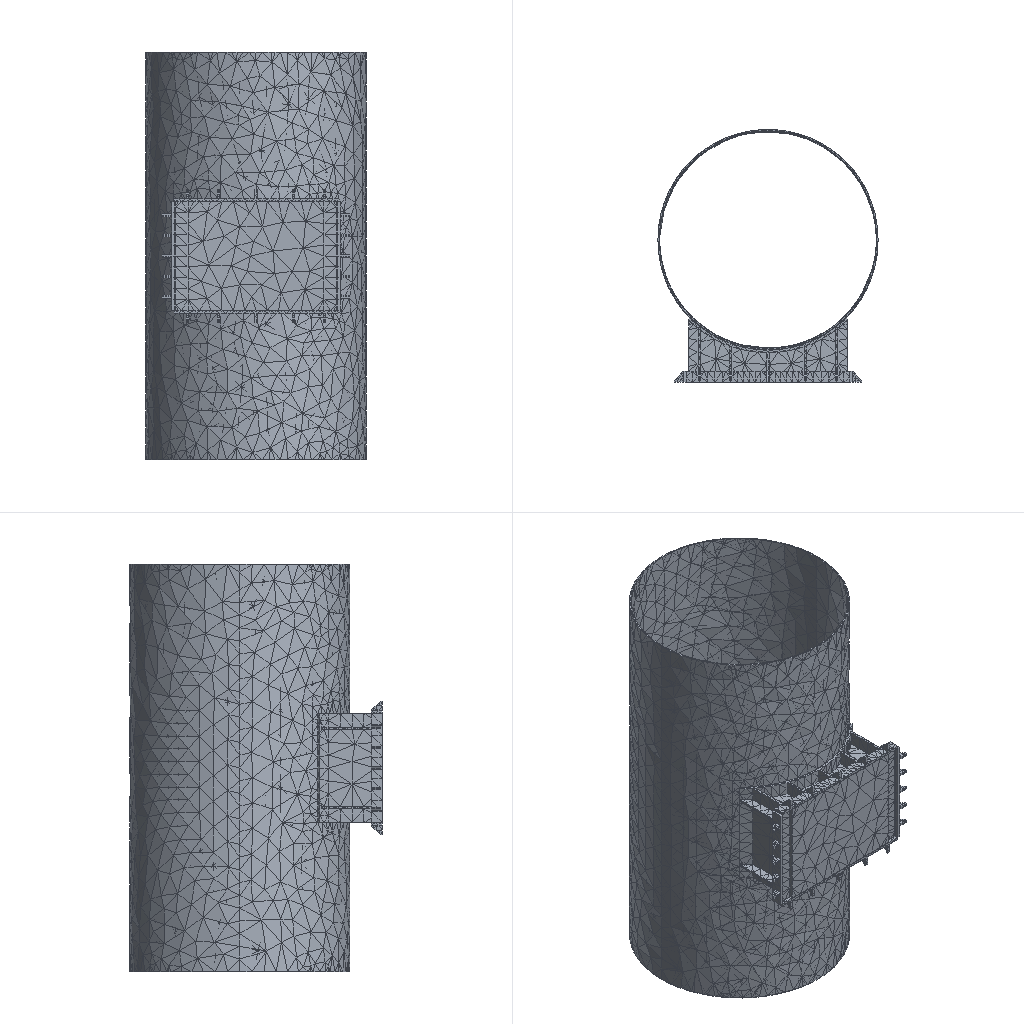Simulation study | ansys workbench
Set-up summary:
category,name,step,type,value,unit,region
solver,ansys_workbench
units,mm-N-s-tonne (MPa),,stated,"/units,MPA"
analysis,LS1,,static
load_step,LS1,LS1,static,nsubst=1; time=1
mesh,nodes,,,24663
mesh,elements,,,11899
element_type,SOLID187,,,9809
element_type,SOLID186,,,594
element_type,SURF154,,,556
element_type,TARGE170,,,470
element_type,CONTA174,,,470
material,q355,,E,200000,tonne s^-2 mm^-1
material,q355,,nu,0.3
material,q355,,density,7.85e-09,tonne mm^-3
material,q355,,conductivity,60.5,tonne mm s^-3 C^-1
material,q355,,specific_heat,4.34e+08,mm^2 s^-2 C^-1
material,q355,,cte,1.2e-05,C^-1
material,q355,,permeability,10000
material,q355,,resistivity,0.00017,ohm mm
load,Define Force Using Surface Effect Elements,LS1,surface-effect pres face 1,7.5,,SURF154 #44
load,Define Force Using Surface Effect Elements,LS1,surface-effect pres face 2,-1.66533e-13,,SURF154 #44
load,Define Force Using Surface Effect Elements,LS1,surface-effect pres face 1,-7.5,,SURF154 #45
load,Define Force Using Surface Effect Elements,LS1,surface-effect pres face 2,-1.66533e-13,,SURF154 #45
load,Define Force Using Surface Effect Elements,LS1,surface-effect pres face 3,-5.493,,SURF154 #46
load,Define Force Using Surface Effect Elements,LS1,surface-effect pres face 3,5.493,,SURF154 #47
load,Define Force Using Surface Effect Elements,LS1,surface-effect pres face 2,-1.574,,SURF154 #48
bc,Fixed Supports,model,fixed,[dofs=ALL],,_FIXEDSU
contact,Contact Region,,bonded (always),element=CONTA174
contact,Contact Region 2,,bonded (always),element=CONTA174
contact,Contact Region 3,,bonded (always),element=CONTA174
contact,Contact Region 4,,bonded (always),element=CONTA174
contact,Contact Region 5,,bonded (always),element=CONTA174
contact,Contact Region 6,,bonded (always),element=CONTA174
contact,Contact Region 7,,bonded (always),element=CONTA174
contact,Contact Region 8,,bonded (always),element=CONTA174
contact,Contact Region 9,,bonded (always),element=CONTA174
contact,Contact Region 10,,bonded (always),element=CONTA174
contact,Contact Region 11,,bonded (always),element=CONTA174
contact,Contact Region 12,,bonded (always),element=CONTA174
contact,Contact Region 13,,bonded (always),element=CONTA174
contact,Contact Region 14,,bonded (always),element=CONTA174
named_set,_FIXEDSU,,node,1393
Ansys APDL input file, long lists of numbers shortened:
/batch
/config,noeldb,1     ! force off writing results to database
*get,_wallstrt,active,,time,wall
! ANSYS input file written by Workbench version 2022 R1
! File used for geometry attach:
/title,wbnew--____ (B5)
! ****** Begin Custom Load Command Snippet ******
/COM, ACT Extensions:
/COM,     LSDYNA, 2021.1
/COM,
! ****** End   Custom Load Command Snippet ******
*DIM,_wb_ProjectScratch_dir,string,248
_wb_ProjectScratch_dir(1) = ''
*DIM,_wb_SolverFiles_dir,string,248
_wb_SolverFiles_dir(1) = ''
*DIM,_wb_userfiles_dir,string,248
_wb_userfiles_dir(1) = ''
/com,--- Data in consistent NMM units. See Solving Units in the help system for more information.
/units,MPA
/nopr
/wb,file,start              !  signify a WB generated input file
/prep7
! Turn off shape checking because checks already performed inside WB mesher.
! See help system for more information.
SHPP,OFF,,NOWARN
/nolist
etcon,set             ! allow ANSYS to choose best KEYOP's for 180x elements, resets any applicable keyopt to MAPDL defaults
/com,*********** Nodes for the whole assembly ***********
nblock,3,,27129
(1i9,3e20.9e3)
        1    -6.344593644E+02    -9.827884966E+02    -3.000000000E+02
! (24662 more lines like these left out)
-1
/wb,elem,start            !  set before creation of elements
/com,*********** Elements for Body 1 "2-FreeParts|__3[3]" ***********
et,1,186
keyo,1,2,1          ! set full integration on SOLID186
eblock,19,solid,,52
(19i9)
        1        1        1        1        0        0        0        0       20        0       63      511      521      513      516      536      526      534      531
! (103 more lines like these left out)
-1
/com,*********** Elements for Body 2 "2-FreeParts|__-__8" ***********
et,2,186
keyo,2,2,1          ! set full integration on SOLID186
eblock,19,solid,,10
(19i9)
        2        2        2        2        0        0        0        0       20        0       53      388      389      390      391      415      414      413      412
! (19 more lines like these left out)
-1
/com,*********** Elements for Body 3 "2-FreeParts|__-__4[2]" ***********
et,3,186
keyo,3,2,1          ! set full integration on SOLID186
eblock,19,solid,,52
(19i9)
        3        3        3        3        0        0        0        0       20        0      115      895      896      901      900      910      909      904      905
! (103 more lines like these left out)
-1
/com,*********** Elements for Body 4 "2-FreeParts|__-__4[1]" ***********
et,4,186
keyo,4,2,1          ! set full integration on SOLID186
eblock,19,solid,,52
(19i9)
        4        4        4        4        0        0        0        0       20        0        1        9       10       15       14       24       23       18       19
! (103 more lines like these left out)
-1
/com,*********** Elements for Body 5 "2-FreeParts|__-__4[4]" ***********
et,5,186
keyo,5,2,1          ! set full integration on SOLID186
eblock,19,solid,,58
(19i9)
        5        5        5        5        0        0        0        0       20        0      413     3064     3065     3082     3073     3101     3100     3083     3092
! (115 more lines like these left out)
-1
/com,*********** Elements for Body 6 "2-FreeParts|__2" ***********
et,6,187
eblock,19,solid,,390
(19i9)
        6        6        6        6        0        0        0        0       10        0      973     5434     5543     5482     5481     5869     6087     5868     5867
! (779 more lines like these left out)
-1
/com,*********** Elements for Body 7 "2-FreeParts|__-__4[5]" ***********
et,7,186
keyo,7,2,1          ! set full integration on SOLID186
eblock,19,solid,,58
(19i9)
        7        7        7        7        0        0        0        0       20        0      471     3476     3477     3494     3485     3513     3512     3495     3504
! (115 more lines like these left out)
-1
/com,*********** Elements for Body 8 "2-FreeParts|__-__4[3]" ***********
et,8,186
keyo,8,2,1          ! set full integration on SOLID186
eblock,19,solid,,52
(19i9)
        8        8        8        8        0        0        0        0       20        0      351     2565     2566     2571     2570     2580     2579     2574     2575
! (103 more lines like these left out)
-1
/com,*********** Elements for Body 9 "2-FreeParts|__3[5]" ***********
et,9,186
keyo,9,2,1          ! set full integration on SOLID186
eblock,19,solid,,66
(19i9)
        9        9        9        9        0        0        0        0       20        0      529     3888     3900     3899     3889     3933     3921     3922     3932
! (131 more lines like these left out)
-1
/com,*********** Elements for Body 10 "2-FreeParts|__3[4]" ***********
et,10,186
keyo,10,2,1          ! set full integration on SOLID186
eblock,19,solid,,66
(19i9)
       10       10       10       10        0        0        0        0       20        0      167     1266     1278     1277     1267     1311     1299     1300     1310
! (131 more lines like these left out)
-1
/com,*********** Elements for Body 11 "2-FreeParts|__-__3" ***********
et,11,187
eblock,19,solid,,378
(19i9)
       11       11       11       11        0        0        0        0       10        0      595     4442     4532     4444     4482     5070     5080     5066     5068
! (755 more lines like these left out)
-1
/com,*********** Elements for Body 12 "2-FreeParts|NONE" ***********
et,12,187
eblock,19,solid,,9041
(19i9)
       12       12       12       12        0        0        0        0       10        0     1363     8461     8464     8850     8818    21356    21383    21362    21360
! (18081 more lines like these left out)
-1
/com,*********** Elements for Body 13 "2-FreeParts|__3[6]" ***********
et,13,186
keyo,13,2,1          ! set full integration on SOLID186
eblock,19,solid,,66
(19i9)
       13       13       13       13        0        0        0        0       20        0      285     2101     2113     2112     2102     2146     2134     2135     2145
! (131 more lines like these left out)
-1
/com,*********** Elements for Body 14 "2-FreeParts|__3[1]" ***********
et,14,186
keyo,14,2,1          ! set full integration on SOLID186
eblock,19,solid,,10
(19i9)
       14       14       14       14        0        0        0        0       20        0      403     2944     2947     2946     2945     2971     2968     2969     2970
! (19 more lines like these left out)
-1
/com,*********** Elements for Body 15 "2-FreeParts|__3[2]" ***********
et,15,186
keyo,15,2,1          ! set full integration on SOLID186
eblock,19,solid,,52
(19i9)
       15       15       15       15        0        0        0        0       20        0      233     1725     1735     1727     1730     1750     1740     1748     1745
! (103 more lines like these left out)
-1
/wb,elem,end               !  done creating elements
/com,*********** Send User Defined Coordinate System(s) ***********
csys,0
toffst,273.15,  ! Temperature offset from absolute zero
/com,*********** Set Reference Temperature ***********
tref,22.
/wb,mat,start              !  starting to send materials
/com,*********** Send Materials ***********
Temperature = 'TEMP' ! Temperature
MP,DENS,1,7.85e-09,	! tonne mm^-3
MP,ALPX,1,1.2e-05,	! C^-1
MP,C,1,434000000,	! mm^2 s^-2 C^-1
MP,KXX,1,60.5,	! tonne mm s^-3 C^-1
MP,RSVX,1,0.00017,	! ohm mm
MP,EX,1,200000,	! tonne s^-2 mm^-1
MP,NUXY,1,0.3,
MP,MURX,1,10000,
Temperature = 'TEMP' ! Temperature
MP,DENS,2,7.85e-09,	! tonne mm^-3
MP,ALPX,2,1.2e-05,	! C^-1
MP,C,2,434000000,	! mm^2 s^-2 C^-1
MP,KXX,2,60.5,	! tonne mm s^-3 C^-1
MP,RSVX,2,0.00017,	! ohm mm
MP,EX,2,200000,	! tonne s^-2 mm^-1
MP,NUXY,2,0.3,
MP,MURX,2,10000,
Temperature = 'TEMP' ! Temperature
MP,DENS,3,7.85e-09,	! tonne mm^-3
MP,ALPX,3,1.2e-05,	! C^-1
MP,C,3,434000000,	! mm^2 s^-2 C^-1
MP,KXX,3,60.5,	! tonne mm s^-3 C^-1
MP,RSVX,3,0.00017,	! ohm mm
MP,EX,3,200000,	! tonne s^-2 mm^-1
MP,NUXY,3,0.3,
MP,MURX,3,10000,
Temperature = 'TEMP' ! Temperature
MP,DENS,4,7.85e-09,	! tonne mm^-3
MP,ALPX,4,1.2e-05,	! C^-1
MP,C,4,434000000,	! mm^2 s^-2 C^-1
MP,KXX,4,60.5,	! tonne mm s^-3 C^-1
MP,RSVX,4,0.00017,	! ohm mm
MP,EX,4,200000,	! tonne s^-2 mm^-1
MP,NUXY,4,0.3,
MP,MURX,4,10000,
Temperature = 'TEMP' ! Temperature
MP,DENS,5,7.85e-09,	! tonne mm^-3
MP,ALPX,5,1.2e-05,	! C^-1
MP,C,5,434000000,	! mm^2 s^-2 C^-1
MP,KXX,5,60.5,	! tonne mm s^-3 C^-1
MP,RSVX,5,0.00017,	! ohm mm
MP,EX,5,200000,	! tonne s^-2 mm^-1
MP,NUXY,5,0.3,
MP,MURX,5,10000,
Temperature = 'TEMP' ! Temperature
MP,DENS,6,7.85e-09,	! tonne mm^-3
MP,ALPX,6,1.2e-05,	! C^-1
MP,C,6,434000000,	! mm^2 s^-2 C^-1
MP,KXX,6,60.5,	! tonne mm s^-3 C^-1
MP,RSVX,6,0.00017,	! ohm mm
MP,EX,6,200000,	! tonne s^-2 mm^-1
MP,NUXY,6,0.3,
MP,MURX,6,10000,
Temperature = 'TEMP' ! Temperature
MP,DENS,7,7.85e-09,	! tonne mm^-3
MP,ALPX,7,1.2e-05,	! C^-1
MP,C,7,434000000,	! mm^2 s^-2 C^-1
MP,KXX,7,60.5,	! tonne mm s^-3 C^-1
MP,RSVX,7,0.00017,	! ohm mm
MP,EX,7,200000,	! tonne s^-2 mm^-1
MP,NUXY,7,0.3,
MP,MURX,7,10000,
Temperature = 'TEMP' ! Temperature
MP,DENS,8,7.85e-09,	! tonne mm^-3
MP,ALPX,8,1.2e-05,	! C^-1
MP,C,8,434000000,	! mm^2 s^-2 C^-1
MP,KXX,8,60.5,	! tonne mm s^-3 C^-1
MP,RSVX,8,0.00017,	! ohm mm
MP,EX,8,200000,	! tonne s^-2 mm^-1
MP,NUXY,8,0.3,
MP,MURX,8,10000,
Temperature = 'TEMP' ! Temperature
MP,DENS,9,7.85e-09,	! tonne mm^-3
MP,ALPX,9,1.2e-05,	! C^-1
MP,C,9,434000000,	! mm^2 s^-2 C^-1
MP,KXX,9,60.5,	! tonne mm s^-3 C^-1
MP,RSVX,9,0.00017,	! ohm mm
MP,EX,9,200000,	! tonne s^-2 mm^-1
MP,NUXY,9,0.3,
MP,MURX,9,10000,
Temperature = 'TEMP' ! Temperature
MP,DENS,10,7.85e-09,	! tonne mm^-3
MP,ALPX,10,1.2e-05,	! C^-1
MP,C,10,434000000,	! mm^2 s^-2 C^-1
MP,KXX,10,60.5,	! tonne mm s^-3 C^-1
MP,RSVX,10,0.00017,	! ohm mm
MP,EX,10,200000,	! tonne s^-2 mm^-1
MP,NUXY,10,0.3,
MP,MURX,10,10000,
Temperature = 'TEMP' ! Temperature
MP,DENS,11,7.85e-09,	! tonne mm^-3
MP,ALPX,11,1.2e-05,	! C^-1
MP,C,11,434000000,	! mm^2 s^-2 C^-1
MP,KXX,11,60.5,	! tonne mm s^-3 C^-1
MP,RSVX,11,0.00017,	! ohm mm
MP,EX,11,200000,	! tonne s^-2 mm^-1
MP,NUXY,11,0.3,
MP,MURX,11,10000,
Temperature = 'TEMP' ! Temperature
MP,DENS,12,7.85e-09,	! tonne mm^-3
MP,ALPX,12,1.2e-05,	! C^-1
MP,C,12,434000000,	! mm^2 s^-2 C^-1
MP,KXX,12,60.5,	! tonne mm s^-3 C^-1
MP,RSVX,12,0.00017,	! ohm mm
MP,EX,12,200000,	! tonne s^-2 mm^-1
MP,NUXY,12,0.3,
MP,MURX,12,10000,
Temperature = 'TEMP' ! Temperature
MP,DENS,13,7.85e-09,	! tonne mm^-3
MP,ALPX,13,1.2e-05,	! C^-1
MP,C,13,434000000,	! mm^2 s^-2 C^-1
MP,KXX,13,60.5,	! tonne mm s^-3 C^-1
MP,RSVX,13,0.00017,	! ohm mm
MP,EX,13,200000,	! tonne s^-2 mm^-1
MP,NUXY,13,0.3,
MP,MURX,13,10000,
Temperature = 'TEMP' ! Temperature
MP,DENS,14,7.85e-09,	! tonne mm^-3
MP,ALPX,14,1.2e-05,	! C^-1
MP,C,14,434000000,	! mm^2 s^-2 C^-1
MP,KXX,14,60.5,	! tonne mm s^-3 C^-1
MP,RSVX,14,0.00017,	! ohm mm
MP,EX,14,200000,	! tonne s^-2 mm^-1
MP,NUXY,14,0.3,
MP,MURX,14,10000,
Temperature = 'TEMP' ! Temperature
MP,DENS,15,7.85e-09,	! tonne mm^-3
MP,ALPX,15,1.2e-05,	! C^-1
MP,C,15,434000000,	! mm^2 s^-2 C^-1
MP,KXX,15,60.5,	! tonne mm s^-3 C^-1
MP,RSVX,15,0.00017,	! ohm mm
MP,EX,15,200000,	! tonne s^-2 mm^-1
MP,NUXY,15,0.3,
MP,MURX,15,10000,
/wb,mat,end                !  done sending materials
!************************* Model Summary ********************
!2-FreeParts|__3[3],	q355,	matid,	1
!2-FreeParts|__-__8,	q355,	matid,	2
!2-FreeParts|__-__4[2],	q355,	matid,	3
!2-FreeParts|__-__4[1],	q355,	matid,	4
!2-FreeParts|__-__4[4],	q355,	matid,	5
!2-FreeParts|__2,	q355,	matid,	6
!2-FreeParts|__-__4[5],	q355,	matid,	7
!2-FreeParts|__-__4[3],	q355,	matid,	8
!2-FreeParts|__3[5],	q355,	matid,	9
!2-FreeParts|__3[4],	q355,	matid,	10
!2-FreeParts|__-__3,	q355,	matid,	11
!2-FreeParts|NONE,	q355,	matid,	12
!2-FreeParts|__3[6],	q355,	matid,	13
!2-FreeParts|__3[1],	q355,	matid,	14
!2-FreeParts|__3[2],	q355,	matid,	15
!************************* End Model Summary ********************
! get the diagonal of the bounding box. Needed later for other things
*get,_xmin,node,,mnloc,x
*get,_ymin,node,,mnloc,y
*get,_zmin,node,,mnloc,z
*get,_xmax,node,,mxloc,x
*get,_ymax,node,,mxloc,y
*get,_zmax,node,,mxloc,z
_ASMDIAG=(_xmax-_xmin)*(_xmax-_xmin)+(_ymax-_ymin)*(_ymax-_ymin)+(_zmax-_zmin)*(_zmax-_zmin)
_ASMDIAG=SQRT(_ASMDIAG)
/wb,contact,start          !  starting to send contact
/com,*********** Create Contact "接触区域" ***********
/com,            Real Constant Set For Above Contact Is 17 & 16
*set,tid,17
*set,cid,16
r,tid
r,cid
et,tid,170
et,cid,174
eblock,10,,,12
(15i9)
    18456       17       17       17        0      603      598      581      580      856      828      826      827
! (11 more lines like these left out)
-1
eblock,10,,,12
(15i9)
    18468       16       16       16        0      603      598      581      580      856      828      826      827
! (11 more lines like these left out)
-1
eblock,10,,,2
(15i9)
    18480       16       17       16        0     2948     2949     2942     2943     3014     3000     2999     3003
    18481       16       17       16        0     2949     2950     2941     2942     3016     2997     2996     3000
-1
eblock,10,,,2
(15i9)
    18482       17       16       17        0     2948     2949     2942     2943     3014     3000     2999     3003
    18483       17       16       17        0     2949     2950     2941     2942     3016     2997     2996     3000
-1
keyo,cid,8,2               ! auto create asymmetric contact (from Program Controlled setting)
keyo,cid,10,0              ! adjust contact stiffness each NR iteration (from Program Controlled setting)
keyo,cid,12,5              ! bonded always
keyo,cid,18,1              ! small sliding turned on by application
keyo,cid,2,0               ! augmented Lagrange (from Program Controlled setting)
keyo,cid,4,0               ! on Gauss point (from Program Controlled setting)
keyo,cid,9,1               ! ignore initial gaps/penetration
keyo,cid,7,0               ! No Prediction
rmod,tid,3,10.      ! FKN
rmod,tid,5,0.       ! ICONT
rmod,tid,6,0.       ! PINB
rmod,tid,10,0.      ! CNOF
rmod,tid,12,0.      ! FKT
rmod,tid,36,68      ! WB DSID
rmod,cid,3,10.      ! FKN
rmod,cid,5,0.       ! ICONT
rmod,cid,6,0.       ! PINB
rmod,cid,10,0.      ! CNOF
rmod,cid,12,0.      ! FKT
rmod,cid,36,68      ! WB DSID
/com,*********** Create Contact "接触区域 2" ***********
/com,            Real Constant Set For Above Contact Is 19 & 18
*set,tid,19
*set,cid,18
r,tid
r,cid
et,tid,170
et,cid,174
eblock,10,,,2
(15i9)
    18484       19       19       19        0      383      382      397      396      431      432      466      435
    18485       19       19       19        0      382      381      398      397      428      429      468      432
-1
eblock,10,,,2
(15i9)
    18486       18       18       18        0      383      382      397      396      431      432      466      435
    18487       18       18       18        0      382      381      398      397      428      429      468      432
-1
eblock,10,,,12
(15i9)
    18488       18       19       18        0      986      977      973      974     1235     1229     1228     1230
! (11 more lines like these left out)
-1
eblock,10,,,12
(15i9)
    18500       19       18       19        0      986      977      973      974     1235     1229     1228     1230
! (11 more lines like these left out)
-1
keyo,cid,8,2               ! auto create asymmetric contact (from Program Controlled setting)
keyo,cid,10,0              ! adjust contact stiffness each NR iteration (from Program Controlled setting)
keyo,cid,12,5              ! bonded always
keyo,cid,18,1              ! small sliding turned on by application
keyo,cid,2,0               ! augmented Lagrange (from Program Controlled setting)
keyo,cid,4,0               ! on Gauss point (from Program Controlled setting)
keyo,cid,9,1               ! ignore initial gaps/penetration
keyo,cid,7,0               ! No Prediction
rmod,tid,3,10.      ! FKN
rmod,tid,5,0.       ! ICONT
rmod,tid,6,0.       ! PINB
rmod,tid,10,0.      ! CNOF
rmod,tid,12,0.      ! FKT
rmod,tid,36,71      ! WB DSID
rmod,cid,3,10.      ! FKN
rmod,cid,5,0.       ! ICONT
rmod,cid,6,0.       ! PINB
rmod,cid,10,0.      ! CNOF
rmod,cid,12,0.      ! FKT
rmod,cid,36,71      ! WB DSID
/com,*********** Create Contact "接触区域 3" ***********
/com,            Real Constant Set For Above Contact Is 21 & 20
*set,tid,21
*set,cid,20
r,tid
r,cid
et,tid,170
et,cid,174
eblock,10,,,2
(15i9)
    18512       21       21       21        0      381      380      399      398      424      425      470      429
    18513       21       21       21        0      380      401      400      399      426      474      472      425
-1
eblock,10,,,2
(15i9)
    18514       20       20       20        0      381      380      399      398      424      425      470      429
    18515       20       20       20        0      380      401      400      399      426      474      472      425
-1
eblock,10,,,12
(15i9)
    18516       20       21       20        0      100       91       87       88      349      343      342      344
! (11 more lines like these left out)
-1
eblock,10,,,12
(15i9)
    18528       21       20       21        0      100       91       87       88      349      343      342      344
! (11 more lines like these left out)
-1
keyo,cid,8,2               ! auto create asymmetric contact (from Program Controlled setting)
keyo,cid,10,0              ! adjust contact stiffness each NR iteration (from Program Controlled setting)
keyo,cid,12,5              ! bonded always
keyo,cid,18,1              ! small sliding turned on by application
keyo,cid,2,0               ! augmented Lagrange (from Program Controlled setting)
keyo,cid,4,0               ! on Gauss point (from Program Controlled setting)
keyo,cid,9,1               ! ignore initial gaps/penetration
keyo,cid,7,0               ! No Prediction
rmod,tid,3,10.      ! FKN
rmod,tid,5,0.       ! ICONT
rmod,tid,6,0.       ! PINB
rmod,tid,10,0.      ! CNOF
rmod,tid,12,0.      ! FKT
rmod,tid,36,74      ! WB DSID
rmod,cid,3,10.      ! FKN
rmod,cid,5,0.       ! ICONT
rmod,cid,6,0.       ! PINB
rmod,cid,10,0.      ! CNOF
rmod,cid,12,0.      ! FKT
rmod,cid,36,74      ! WB DSID
/com,*********** Create Contact "接触区域 4" ***********
/com,            Real Constant Set For Above Contact Is 23 & 22
*set,tid,23
*set,cid,22
r,tid
r,cid
et,tid,170
et,cid,174
eblock,10,,,2
(15i9)
    18540       23       23       23        0      389      388      391      390      449      450      454      452
    18541       23       23       23        0      388      387      392      391      446      447      456      450
-1
eblock,10,,,2
(15i9)
    18542       22       22       22        0      389      388      391      390      449      450      454      452
    18543       22       22       22        0      388      387      392      391      446      447      456      450
-1
eblock,10,,,12
(15i9)
    18544       22       23       22        0     3172     3163     3157     3158     3445     3436     3435     3437
! (11 more lines like these left out)
-1
eblock,10,,,12
(15i9)
    18556       23       22       23        0     3172     3163     3157     3158     3445     3436     3435     3437
! (11 more lines like these left out)
-1
keyo,cid,8,2               ! auto create asymmetric contact (from Program Controlled setting)
keyo,cid,10,0              ! adjust contact stiffness each NR iteration (from Program Controlled setting)
keyo,cid,12,5              ! bonded always
keyo,cid,18,1              ! small sliding turned on by application
keyo,cid,2,0               ! augmented Lagrange (from Program Controlled setting)
keyo,cid,4,0               ! on Gauss point (from Program Controlled setting)
keyo,cid,9,1               ! ignore initial gaps/penetration
keyo,cid,7,0               ! No Prediction
rmod,tid,3,10.      ! FKN
rmod,tid,5,0.       ! ICONT
rmod,tid,6,0.       ! PINB
rmod,tid,10,0.      ! CNOF
rmod,tid,12,0.      ! FKT
rmod,tid,36,77      ! WB DSID
rmod,cid,3,10.      ! FKN
rmod,cid,5,0.       ! ICONT
rmod,cid,6,0.       ! PINB
rmod,cid,10,0.      ! CNOF
rmod,cid,12,0.      ! FKT
rmod,cid,36,77      ! WB DSID
/com,*********** Create Contact "接触区域 5" ***********
/com,            Real Constant Set For Above Contact Is 25 & 24
*set,tid,25
*set,cid,24
r,tid
r,cid
et,tid,170
et,cid,174
eblock,10,,,2
(15i9)
    18568       25       25       25        0      387      386      393      392      443      444      458      447
    18569       25       25       25        0      386      385      394      393      440      441      460      444
-1
eblock,10,,,2
(15i9)
    18570       24       24       24        0      387      386      393      392      443      444      458      447
    18571       24       24       24        0      386      385      394      393      440      441      460      444
-1
eblock,10,,,12
(15i9)
    18572       24       25       24        0     3584     3575     3569     3570     3857     3848     3847     3849
! (11 more lines like these left out)
-1
eblock,10,,,12
(15i9)
    18584       25       24       25        0     3584     3575     3569     3570     3857     3848     3847     3849
! (11 more lines like these left out)
-1
keyo,cid,8,2               ! auto create asymmetric contact (from Program Controlled setting)
keyo,cid,10,0              ! adjust contact stiffness each NR iteration (from Program Controlled setting)
keyo,cid,12,5              ! bonded always
keyo,cid,18,1              ! small sliding turned on by application
keyo,cid,2,0               ! augmented Lagrange (from Program Controlled setting)
keyo,cid,4,0               ! on Gauss point (from Program Controlled setting)
keyo,cid,9,1               ! ignore initial gaps/penetration
keyo,cid,7,0               ! No Prediction
rmod,tid,3,10.      ! FKN
rmod,tid,5,0.       ! ICONT
rmod,tid,6,0.       ! PINB
rmod,tid,10,0.      ! CNOF
rmod,tid,12,0.      ! FKT
rmod,tid,36,80      ! WB DSID
rmod,cid,3,10.      ! FKN
rmod,cid,5,0.       ! ICONT
rmod,cid,6,0.       ! PINB
rmod,cid,10,0.      ! CNOF
rmod,cid,12,0.      ! FKT
rmod,cid,36,80      ! WB DSID
/com,*********** Create Contact "接触区域 6" ***********
/com,            Real Constant Set For Above Contact Is 27 & 26
*set,tid,27
*set,cid,26
r,tid
r,cid
et,tid,170
et,cid,174
eblock,10,,,2
(15i9)
    18596       27       27       27        0      385      384      395      394      437      438      462      441
    18597       27       27       27        0      384      383      396      395      434      435      464      438
-1
eblock,10,,,2
(15i9)
    18598       26       26       26        0      385      384      395      394      437      438      462      441
    18599       26       26       26        0      384      383      396      395      434      435      464      438
-1
eblock,10,,,12
(15i9)
    18600       26       27       26        0     2656     2647     2643     2644     2905     2899     2898     2900
! (11 more lines like these left out)
-1
eblock,10,,,12
(15i9)
    18612       27       26       27        0     2656     2647     2643     2644     2905     2899     2898     2900
! (11 more lines like these left out)
-1
keyo,cid,8,2               ! auto create asymmetric contact (from Program Controlled setting)
keyo,cid,10,0              ! adjust contact stiffness each NR iteration (from Program Controlled setting)
keyo,cid,12,5              ! bonded always
keyo,cid,18,1              ! small sliding turned on by application
keyo,cid,2,0               ! augmented Lagrange (from Program Controlled setting)
keyo,cid,4,0               ! on Gauss point (from Program Controlled setting)
keyo,cid,9,1               ! ignore initial gaps/penetration
keyo,cid,7,0               ! No Prediction
rmod,tid,3,10.      ! FKN
rmod,tid,5,0.       ! ICONT
rmod,tid,6,0.       ! PINB
rmod,tid,10,0.      ! CNOF
rmod,tid,12,0.      ! FKT
rmod,tid,36,83      ! WB DSID
rmod,cid,3,10.      ! FKN
rmod,cid,5,0.       ! ICONT
rmod,cid,6,0.       ! PINB
rmod,cid,10,0.      ! CNOF
rmod,cid,12,0.      ! FKT
rmod,cid,36,83      ! WB DSID
/com,*********** Create Contact "接触区域 7" ***********
/com,            Real Constant Set For Above Contact Is 29 & 28
*set,tid,29
*set,cid,28
r,tid
r,cid
et,tid,170
et,cid,174
eblock,10,,,10
(15i9)
    18624       29       29       29        0      412      415      414      413      497      499      498      496
! (9 more lines like these left out)
-1
eblock,10,,,10
(15i9)
    18634       28       28       28        0      412      415      414      413      497      499      498      496
! (9 more lines like these left out)
-1
eblock,10,,,50
(15i9)
    18644       28       29       28        0     7464     6813     7255     7255    12286    12285     7255    15039
! (49 more lines like these left out)
-1
eblock,10,,,50
(15i9)
    18694       29       28       29        0     7464     6813     7255     7255    12286    12285     7255    15039
! (49 more lines like these left out)
-1
keyo,cid,8,2               ! auto create asymmetric contact (from Program Controlled setting)
keyo,cid,10,0              ! adjust contact stiffness each NR iteration (from Program Controlled setting)
keyo,cid,12,5              ! bonded always
keyo,cid,18,1              ! small sliding turned on by application
keyo,cid,2,0               ! augmented Lagrange (from Program Controlled setting)
keyo,cid,4,0               ! on Gauss point (from Program Controlled setting)
keyo,cid,9,1               ! ignore initial gaps/penetration
keyo,cid,7,0               ! No Prediction
rmod,tid,3,10.      ! FKN
rmod,tid,5,0.       ! ICONT
rmod,tid,6,0.       ! PINB
rmod,tid,10,0.      ! CNOF
rmod,tid,12,0.      ! FKT
rmod,tid,36,86      ! WB DSID
rmod,cid,3,10.      ! FKN
rmod,cid,5,0.       ! ICONT
rmod,cid,6,0.       ! PINB
rmod,cid,10,0.      ! CNOF
rmod,cid,12,0.      ! FKT
rmod,cid,36,86      ! WB DSID
/com,*********** Create Contact "接触区域 8" ***********
/com,            Real Constant Set For Above Contact Is 31 & 30
*set,tid,31
*set,cid,30
r,tid
r,cid
et,tid,170
et,cid,174
eblock,10,,,50
(15i9)
    18744       31       31       31        0     5529     5459     5422     5422     6001     5794     5422     5798
! (49 more lines like these left out)
-1
eblock,10,,,50
(15i9)
    18794       30       30       30        0     5529     5459     5422     5422     6001     5794     5422     5798
! (49 more lines like these left out)
-1
eblock,10,,,55
(15i9)
    18844       30       31       30        0     6649     6899     7521     7521    11018    12914     7521    11023
! (54 more lines like these left out)
-1
eblock,10,,,55
(15i9)
    18899       31       30       31        0     6649     6899     7521     7521    11018    12914     7521    11023
! (54 more lines like these left out)
-1
keyo,cid,8,2               ! auto create asymmetric contact (from Program Controlled setting)
keyo,cid,10,0              ! adjust contact stiffness each NR iteration (from Program Controlled setting)
keyo,cid,12,5              ! bonded always
keyo,cid,18,1              ! small sliding turned on by application
keyo,cid,2,0               ! augmented Lagrange (from Program Controlled setting)
keyo,cid,4,0               ! on Gauss point (from Program Controlled setting)
keyo,cid,9,1               ! ignore initial gaps/penetration
keyo,cid,7,0               ! No Prediction
rmod,tid,3,10.      ! FKN
rmod,tid,5,0.       ! ICONT
rmod,tid,6,0.       ! PINB
rmod,tid,10,0.      ! CNOF
rmod,tid,12,0.      ! FKT
rmod,tid,36,89      ! WB DSID
rmod,cid,3,10.      ! FKN
rmod,cid,5,0.       ! ICONT
rmod,cid,6,0.       ! PINB
rmod,cid,10,0.      ! CNOF
rmod,cid,12,0.      ! FKT
rmod,cid,36,89      ! WB DSID
/com,*********** Create Contact "接触区域 9" ***********
/com,            Real Constant Set For Above Contact Is 33 & 32
*set,tid,33
*set,cid,32
r,tid
r,cid
et,tid,170
et,cid,174
eblock,10,,,12
(15i9)
    18954       33       33       33        0     4004     3999     3990     3989     4313     4297     4295     4296
! (11 more lines like these left out)
-1
eblock,10,,,12
(15i9)
    18966       32       32       32        0     4004     3999     3990     3989     4313     4297     4295     4296
! (11 more lines like these left out)
-1
eblock,10,,,2
(15i9)
    18978       32       33       32        0     2952     2953     2938     2939     3022     2988     2987     2991
    18979       32       33       32        0     2953     2954     2937     2938     3024     2985     2984     2988
-1
eblock,10,,,2
(15i9)
    18980       33       32       33        0     2952     2953     2938     2939     3022     2988     2987     2991
    18981       33       32       33        0     2953     2954     2937     2938     3024     2985     2984     2988
-1
keyo,cid,8,2               ! auto create asymmetric contact (from Program Controlled setting)
keyo,cid,10,0              ! adjust contact stiffness each NR iteration (from Program Controlled setting)
keyo,cid,12,5              ! bonded always
keyo,cid,18,1              ! small sliding turned on by application
keyo,cid,2,0               ! augmented Lagrange (from Program Controlled setting)
keyo,cid,4,0               ! on Gauss point (from Program Controlled setting)
keyo,cid,9,1               ! ignore initial gaps/penetration
keyo,cid,7,0               ! No Prediction
rmod,tid,3,10.      ! FKN
rmod,tid,5,0.       ! ICONT
rmod,tid,6,0.       ! PINB
rmod,tid,10,0.      ! CNOF
rmod,tid,12,0.      ! FKT
rmod,tid,36,92      ! WB DSID
rmod,cid,3,10.      ! FKN
rmod,cid,5,0.       ! ICONT
rmod,cid,6,0.       ! PINB
rmod,cid,10,0.      ! CNOF
rmod,cid,12,0.      ! FKT
rmod,cid,36,92      ! WB DSID
/com,*********** Create Contact "接触区域 10" ***********
/com,            Real Constant Set For Above Contact Is 35 & 34
*set,tid,35
*set,cid,34
r,tid
r,cid
et,tid,170
et,cid,174
eblock,10,,,12
(15i9)
    18982       35       35       35        0     1382     1377     1368     1367     1691     1675     1673     1674
! (11 more lines like these left out)
-1
eblock,10,,,12
(15i9)
    18994       34       34       34        0     1382     1377     1368     1367     1691     1675     1673     1674
! (11 more lines like these left out)
-1
eblock,10,,,2
(15i9)
    19006       34       35       34        0     2950     2951     2940     2941     3018     2994     2993     2997
    19007       34       35       34        0     2951     2952     2939     2940     3020     2991     2990     2994
-1
eblock,10,,,2
(15i9)
    19008       35       34       35        0     2950     2951     2940     2941     3018     2994     2993     2997
    19009       35       34       35        0     2951     2952     2939     2940     3020     2991     2990     2994
-1
keyo,cid,8,2               ! auto create asymmetric contact (from Program Controlled setting)
keyo,cid,10,0              ! adjust contact stiffness each NR iteration (from Program Controlled setting)
keyo,cid,12,5              ! bonded always
keyo,cid,18,1              ! small sliding turned on by application
keyo,cid,2,0               ! augmented Lagrange (from Program Controlled setting)
keyo,cid,4,0               ! on Gauss point (from Program Controlled setting)
keyo,cid,9,1               ! ignore initial gaps/penetration
keyo,cid,7,0               ! No Prediction
rmod,tid,3,10.      ! FKN
rmod,tid,5,0.       ! ICONT
rmod,tid,6,0.       ! PINB
rmod,tid,10,0.      ! CNOF
rmod,tid,12,0.      ! FKT
rmod,tid,36,95      ! WB DSID
rmod,cid,3,10.      ! FKN
rmod,cid,5,0.       ! ICONT
rmod,cid,6,0.       ! PINB
rmod,cid,10,0.      ! CNOF
rmod,cid,12,0.      ! FKT
rmod,cid,36,95      ! WB DSID
/com,*********** Create Contact "接触区域 11" ***********
/com,            Real Constant Set For Above Contact Is 37 & 36
*set,tid,37
*set,cid,36
r,tid
r,cid
et,tid,170
et,cid,174
eblock,10,,,50
(15i9)
    19010       37       37       37        0     4380     4486     4528     4528     4779     5228     4528     4781
! (49 more lines like these left out)
-1
eblock,10,,,50
(15i9)
    19060       36       36       36        0     4380     4486     4528     4528     4779     5228     4528     4781
! (49 more lines like these left out)
-1
eblock,10,,,55
(15i9)
    19110       36       37       36        0     6655     7530     6904     6904    11072    12934     6904    11067
! (54 more lines like these left out)
-1
eblock,10,,,55
(15i9)
    19165       37       36       37        0     6655     7530     6904     6904    11072    12934     6904    11067
! (54 more lines like these left out)
-1
keyo,cid,8,2               ! auto create asymmetric contact (from Program Controlled setting)
keyo,cid,10,0              ! adjust contact stiffness each NR iteration (from Program Controlled setting)
keyo,cid,12,5              ! bonded always
keyo,cid,18,1              ! small sliding turned on by application
keyo,cid,2,0               ! augmented Lagrange (from Program Controlled setting)
keyo,cid,4,0               ! on Gauss point (from Program Controlled setting)
keyo,cid,9,1               ! ignore initial gaps/penetration
keyo,cid,7,0               ! No Prediction
rmod,tid,3,10.      ! FKN
rmod,tid,5,0.       ! ICONT
rmod,tid,6,0.       ! PINB
rmod,tid,10,0.      ! CNOF
rmod,tid,12,0.      ! FKT
rmod,tid,36,98      ! WB DSID
rmod,cid,3,10.      ! FKN
rmod,cid,5,0.       ! ICONT
rmod,cid,6,0.       ! PINB
rmod,cid,10,0.      ! CNOF
rmod,cid,12,0.      ! FKT
rmod,cid,36,98      ! WB DSID
/com,*********** Create Contact "接触区域 12" ***********
/com,            Real Constant Set For Above Contact Is 39 & 38
*set,tid,39
*set,cid,38
r,tid
r,cid
et,tid,170
et,cid,174
eblock,10,,,50
(15i9)
    19220       39       39       39        0     6604     6788     7434     7434    10647    12106     7434    10651
! (49 more lines like these left out)
-1
eblock,10,,,50
(15i9)
    19270       38       38       38        0     6604     6788     7434     7434    10647    12106     7434    10651
! (49 more lines like these left out)
-1
eblock,10,,,10
(15i9)
    19320       38       39       38        0     2971     2968     2969     2970     3053     3052     3054     3055
! (9 more lines like these left out)
-1
eblock,10,,,10
(15i9)
    19330       39       38       39        0     2971     2968     2969     2970     3053     3052     3054     3055
! (9 more lines like these left out)
-1
keyo,cid,8,2               ! auto create asymmetric contact (from Program Controlled setting)
keyo,cid,10,0              ! adjust contact stiffness each NR iteration (from Program Controlled setting)
keyo,cid,12,5              ! bonded always
keyo,cid,18,1              ! small sliding turned on by application
keyo,cid,2,0               ! augmented Lagrange (from Program Controlled setting)
keyo,cid,4,0               ! on Gauss point (from Program Controlled setting)
keyo,cid,9,1               ! ignore initial gaps/penetration
keyo,cid,7,0               ! No Prediction
rmod,tid,3,10.      ! FKN
rmod,tid,5,0.       ! ICONT
rmod,tid,6,0.       ! PINB
rmod,tid,10,0.      ! CNOF
rmod,tid,12,0.      ! FKT
rmod,tid,36,101     ! WB DSID
rmod,cid,3,10.      ! FKN
rmod,cid,5,0.       ! ICONT
rmod,cid,6,0.       ! PINB
rmod,cid,10,0.      ! CNOF
rmod,cid,12,0.      ! FKT
rmod,cid,36,101     ! WB DSID
/com,*********** Create Contact "接触区域 13" ***********
/com,            Real Constant Set For Above Contact Is 41 & 40
*set,tid,41
*set,cid,40
r,tid
r,cid
et,tid,170
et,cid,174
eblock,10,,,12
(15i9)
    19340       41       41       41        0     2217     2212     2203     2202     2526     2510     2508     2509
! (11 more lines like these left out)
-1
eblock,10,,,12
(15i9)
    19352       40       40       40        0     2217     2212     2203     2202     2526     2510     2508     2509
! (11 more lines like these left out)
-1
eblock,10,,,2
(15i9)
    19364       40       41       40        0     2954     2955     2936     2937     3026     2981     2980     2985
    19365       40       41       40        0     2955     2956     2957     2936     3028     3030     2982     2981
-1
eblock,10,,,2
(15i9)
    19366       41       40       41        0     2954     2955     2936     2937     3026     2981     2980     2985
    19367       41       40       41        0     2955     2956     2957     2936     3028     3030     2982     2981
-1
keyo,cid,8,2               ! auto create asymmetric contact (from Program Controlled setting)
keyo,cid,10,0              ! adjust contact stiffness each NR iteration (from Program Controlled setting)
keyo,cid,12,5              ! bonded always
keyo,cid,18,1              ! small sliding turned on by application
keyo,cid,2,0               ! augmented Lagrange (from Program Controlled setting)
keyo,cid,4,0               ! on Gauss point (from Program Controlled setting)
keyo,cid,9,1               ! ignore initial gaps/penetration
keyo,cid,7,0               ! No Prediction
rmod,tid,3,10.      ! FKN
rmod,tid,5,0.       ! ICONT
rmod,tid,6,0.       ! PINB
rmod,tid,10,0.      ! CNOF
rmod,tid,12,0.      ! FKT
rmod,tid,36,104     ! WB DSID
rmod,cid,3,10.      ! FKN
rmod,cid,5,0.       ! ICONT
rmod,cid,6,0.       ! PINB
rmod,cid,10,0.      ! CNOF
rmod,cid,12,0.      ! FKT
rmod,cid,36,104     ! WB DSID
/com,*********** Create Contact "接触区域 14" ***********
/com,            Real Constant Set For Above Contact Is 43 & 42
*set,tid,43
*set,cid,42
r,tid
r,cid
et,tid,170
et,cid,174
eblock,10,,,2
(15i9)
    19368       43       43       43        0     2946     2947     2944     2945     3010     3006     3005     3008
    19369       43       43       43        0     2947     2948     2943     2944     3012     3003     3002     3006
-1
eblock,10,,,2
(15i9)
    19370       42       42       42        0     2946     2947     2944     2945     3010     3006     3005     3008
    19371       42       42       42        0     2947     2948     2943     2944     3012     3003     3002     3006
-1
eblock,10,,,12
(15i9)
    19372       42       43       42        0     1817     1812     1795     1794     2070     2042     2040     2041
! (11 more lines like these left out)
-1
eblock,10,,,12
(15i9)
    19384       43       42       43        0     1817     1812     1795     1794     2070     2042     2040     2041
! (11 more lines like these left out)
-1
keyo,cid,8,2               ! auto create asymmetric contact (from Program Controlled setting)
keyo,cid,10,0              ! adjust contact stiffness each NR iteration (from Program Controlled setting)
keyo,cid,12,5              ! bonded always
keyo,cid,18,1              ! small sliding turned on by application
keyo,cid,2,0               ! augmented Lagrange (from Program Controlled setting)
keyo,cid,4,0               ! on Gauss point (from Program Controlled setting)
keyo,cid,9,1               ! ignore initial gaps/penetration
keyo,cid,7,0               ! No Prediction
rmod,tid,3,10.      ! FKN
rmod,tid,5,0.       ! ICONT
rmod,tid,6,0.       ! PINB
rmod,tid,10,0.      ! CNOF
rmod,tid,12,0.      ! FKT
rmod,tid,36,107     ! WB DSID
rmod,cid,3,10.      ! FKN
rmod,cid,5,0.       ! ICONT
rmod,cid,6,0.       ! PINB
rmod,cid,10,0.      ! CNOF
rmod,cid,12,0.      ! FKT
rmod,cid,36,107     ! WB DSID
nsel,all
esel,all
/wb,contact,end            !  done creating contacts
/golist
/wb,load,start             !  starting to send loads
/com,*********** Fixed Supports ***********
CMBLOCK,_FIXEDSU,NODE,     1393
(8i10)
        64        65        66        67        68        69        70        71
! (174 more lines like these left out)
cmsel,s,_FIXEDSU
d,all,all
nsel,all
/com,*********** Define Force Using Surface Effect Elements ***********
local,12,0,0.,0.,0.,0.,0.,0.
csys,0
et,44,154
eblock,10,,,36
(15i9)
    19396       44       44       44       12     7464     6813     7255     7255    12286    12285     7255    15039
! (35 more lines like these left out)
-1
esel,s,type,,44
keyop,44,2,1                ! Apply load in local coordinate system
keyop,44,7,1                ! Use original area so load is constant in large deformation
esel,all
/com,*********** Define Force Using Surface Effect Elements ***********
local,13,0,0.,0.,0.,0.,0.,0.
csys,0
et,45,154
eblock,10,,,36
(15i9)
    19432       45       45       45       13     6604     6788     7434     7434    10647    12106     7434    10651
! (35 more lines like these left out)
-1
esel,s,type,,45
keyop,45,2,1                ! Apply load in local coordinate system
keyop,45,7,1                ! Use original area so load is constant in large deformation
esel,all
/com,*********** Define Force Using Surface Effect Elements ***********
local,14,0,0.,0.,0.,0.,0.,0.
csys,0
et,46,154
eblock,10,,,176
(15i9)
    19468       46       46       46       14     6679     7305     7105     7105    11271    14299     7105    11269
! (175 more lines like these left out)
-1
esel,s,type,,46
keyop,46,2,1                ! Apply load in local coordinate system
keyop,46,7,1                ! Use original area so load is constant in large deformation
esel,all
/com,*********** Define Force Using Surface Effect Elements ***********
local,15,0,0.,0.,0.,0.,0.,0.
csys,0
et,47,154
eblock,10,,,176
(15i9)
    19644       47       47       47       15     6693     7319     7507     7507    11379    15426     7507    11381
! (175 more lines like these left out)
-1
esel,s,type,,47
keyop,47,2,1                ! Apply load in local coordinate system
keyop,47,7,1                ! Use original area so load is constant in large deformation
esel,all
/com,*********** Define Force Using Surface Effect Elements ***********
local,16,0,0.,0.,0.,0.,0.,0.
csys,0
et,48,154
eblock,10,,,132
(15i9)
    19820       48       48       48       16     6814     7460     7468     7468    12294    16024     7468    12295
! (131 more lines like these left out)
-1
esel,s,type,,48
keyop,48,2,1                ! Apply load in local coordinate system
keyop,48,7,1                ! Use original area so load is constant in large deformation
esel,all
/gst,on,on
fini
*get,_numnode,node,0,count
*get,_numelem,elem,0,count
*get, _MAXELEMNUM, elem, 0, NUM, MAX
*get, _MAXNODENUM, node, 0, NUM, MAX
*get, _MAXELEMTYPE, etyp, 0, NUM, MAX
*get, _MAXREALCONST, real, 0, NUM, MAX
/go
/wb,load,end               !  done creating loads
/com,--- Number of total nodes = %_numnode%
/com,--- Number of contact elements = 1496
/com,--- Number of spring elements = 0
/com,--- Number of bearing elements = 0
/com,--- Number of solid elements = 10403
/com,--- Number of condensed parts = 0
/com,--- Number of total elements = %_numelem%
*get,_wallbsol,active,,time,wall
/com,****************************************************************************
/com,*************************    SOLUTION       ********************************
/com,****************************************************************************
/solu
antype,0                   ! static analysis
_thickRatio=  0     ! Ratio of thick parts in the model
eqsl,sparse,,,,,1
cntr,print,1               ! print out contact info and also make no initial contact an error
dmpoption,emat,no             ! Don't combine emat file for DANSYS
dmpoption,esav,no             ! Don't combine esav file for DANSYS
nldiag,cont,iter           ! print out contact info each equilibrium iteration
rescontrol,,none                 ! Do not keep any restart files
/com,****************************************************
/com,******************* SOLVE FOR LS 1 OF 1 ****************
esel,s,type,,44
nsle
sfe,all,1,pres,1,7.5
sfe,all,2,pres,1,-1.66533453693774e-013
sfe,all,3,pres,1,0.
esel,s,type,,45
nsle
sfe,all,1,pres,1,-7.5
sfe,all,2,pres,1,-1.66533453693774e-013
sfe,all,3,pres,1,0.
esel,s,type,,46
nsle
sfe,all,1,pres,1,0.
sfe,all,2,pres,1,0.
sfe,all,3,pres,1,-5.493
esel,s,type,,47
nsle
sfe,all,1,pres,1,0.
sfe,all,2,pres,1,0.
sfe,all,3,pres,1,5.493
esel,s,type,,48
nsle
sfe,all,1,pres,1,0.
sfe,all,2,pres,1,-1.574
sfe,all,3,pres,1,0.
nsel,all
esel,all
/nopr
/gopr
nsub,1,1,1
time,1.
outres,erase
outres,all,none
outres,nsol,all,
outres,rsol,all
outres,eangl,all
outres,etmp,all
outres,veng,all
outres,strs,all,
outres,epel,all,
outres,eppl,all,
outres,cont,all,
! *********** WB SOLVE COMMAND ***********
! check interactive state
*get,ANSINTER_,active,,int
*if,ANSINTER_,ne,0,then
/eof
*endif
solve
/com *************** Write FE CONNECTORS *********
CEWRITE,file,ce,,INTE
/com,****************************************************
/com,*************** FINISHED SOLVE FOR LS 1 *************
*get,_wallasol,active,,time,wall
/nopr
*get,_numnode,node,0,count
*get,_numelem,elem,0,count
*get, _MAXELEMNUM, elem, 0, NUM, MAX
*get, _MAXNODENUM, node, 0, NUM, MAX,,,INTERNAL
*get, _MAXELEMTYPE, etyp, 0, NUM, MAX
*get, _MAXREALCONST, real, 0, NUM, MAX
/gopr
/post1
xmlo,ENCODING,ISO-8859-1
xmlo,parm
/xml,parm,xml
fini
/gopr
*get,_walldone,active,,time,wall
_preptime=(_wallbsol-_wallstrt)*3600
_solvtime=(_wallasol-_wallbsol)*3600
_posttime=(_walldone-_wallasol)*3600
_totaltim=(_walldone-_wallstrt)*3600
*get,_dlbratio,active,0,solu,dlbr
*get,_combtime,active,0,solu,comb
*get,_ssmode,active,0,solu,ssmm
*get,_ndofs,active,0,solu,ndof
*get,_sol_end_time,active,0,set,time
*if,_sol_end_time,eq,1.,then
/fclean				!clean distributed files
*endif
/com,--- Total number of nodes = %_numnode%
/com,--- Total number of elements = %_numelem%
/com,--- Element load balance ratio = %_dlbratio%
/com,--- Time to combine distributed files = %_combtime%
/com,--- Sparse memory mode = %_ssmode%
/com,--- Number of DOF = %_ndofs%
/wb,file,end               ! done with WB generated input
Results summary:
result,analyses[0].index,,,1
result,analyses[0].system,,,SYS
result,analyses[0].deck,,,deck.dat
result,analyses[0].solve_status,,,completed
result,analyses[0].analysis_type,,,static
result,analyses[0].physics,,,mechanical
result,analyses[0].unit_system,,,"NMM: mm, ton, N, s, mV, mA, degC"
result,analyses[0].n_sets,,,1
result,analyses[0].load_steps[0].set,set=1,,1
result,analyses[0].load_steps[0].time_or_freq,set=1,,1
result,analyses[0].load_steps[0].max_displacement_magnitude,set=1,,0.02649
result,analyses[0].load_steps[0].max_von_mises_nodal,set=1,,62.649
result,analyses[0].load_steps[0].reaction_force_sum_xyz[1],set=1,,6.02802e-06
result,analyses[0].load_steps[0].reaction_force_sum_xyz[2],set=1,,500000
result,analyses[0].load_steps[0].reaction_force_sum_xyz[3],set=1,,8.59847e-05